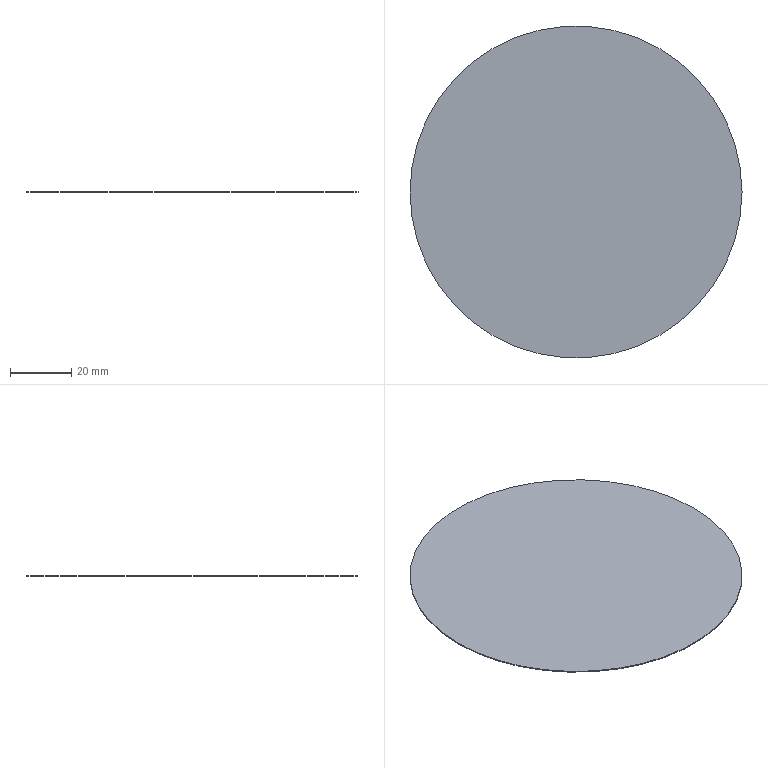Part | SolidWorks | features Extrusion 1 | 1 solid | 4 faces | box 108 x 108 x 0.3 mm | volume 2748 mm3 | cylinder 2 | plane 2 | commonest cylinder face diameters 108 x2
STEP:
#1=CARTESIAN_POINT('',(54.,0.,0.3));
#2=VERTEX_POINT('',#1);
#3=CARTESIAN_POINT('',(-54.,0.,0.3));
#4=VERTEX_POINT('',#3);
#5=CARTESIAN_POINT('',(0.,0.,0.3));
#6=DIRECTION('',(0.,0.,1.));
#7=DIRECTION('',(1.,0.,0.));
#8=AXIS2_PLACEMENT_3D('',#5,#6,#7);
#9=CIRCLE('',#8,54.);
#10=EDGE_CURVE('',#2,#4,#9,.T.);
#11=ORIENTED_EDGE('',*,*,#10,.F.);
#12=CARTESIAN_POINT('',(54.,0.,0.));
#13=VERTEX_POINT('',#12);
#14=CARTESIAN_POINT('',(54.,0.,0.3));
#15=DIRECTION('',(0.,0.,-1.));
#16=VECTOR('',#15,1000.);
#17=LINE('',#14,#16);
#18=EDGE_CURVE('',#2,#13,#17,.T.);
#19=ORIENTED_EDGE('',*,*,#18,.T.);
#20=CARTESIAN_POINT('',(-54.,0.,0.));
#21=VERTEX_POINT('',#20);
#22=CARTESIAN_POINT('',(0.,0.,0.));
#23=DIRECTION('',(0.,0.,1.));
#24=DIRECTION('',(1.,0.,0.));
#25=AXIS2_PLACEMENT_3D('',#22,#23,#24);
#26=CIRCLE('',#25,54.);
#27=EDGE_CURVE('',#13,#21,#26,.T.);
#28=ORIENTED_EDGE('',*,*,#27,.T.);
#29=CARTESIAN_POINT('',(-54.,0.,0.3));
#30=DIRECTION('',(0.,0.,-1.));
#31=VECTOR('',#30,1000.);
#32=LINE('',#29,#31);
#33=EDGE_CURVE('',#4,#21,#32,.T.);
#34=ORIENTED_EDGE('',*,*,#33,.F.);
#35=EDGE_LOOP('',(#11,#19,#28,#34));
#36=FACE_OUTER_BOUND('',#35,.T.);
#37=CARTESIAN_POINT('',(0.,0.,0.3));
#38=DIRECTION('',(0.,0.,-1.));
#39=DIRECTION('',(-1.,0.,0.));
#40=AXIS2_PLACEMENT_3D('',#37,#38,#39);
#41=CYLINDRICAL_SURFACE('',#40,54.);
#42=ADVANCED_FACE('',(#36),#41,.T.);
#43=ORIENTED_EDGE('',*,*,#18,.F.);
#44=CARTESIAN_POINT('',(0.,0.,0.3));
#45=DIRECTION('',(0.,0.,1.));
#46=DIRECTION('',(1.,0.,0.));
#47=AXIS2_PLACEMENT_3D('',#44,#45,#46);
#48=CIRCLE('',#47,54.);
#49=EDGE_CURVE('',#4,#2,#48,.T.);
#50=ORIENTED_EDGE('',*,*,#49,.F.);
#51=ORIENTED_EDGE('',*,*,#33,.T.);
#52=CARTESIAN_POINT('',(0.,0.,0.));
#53=DIRECTION('',(0.,0.,1.));
#54=DIRECTION('',(1.,0.,0.));
#55=AXIS2_PLACEMENT_3D('',#52,#53,#54);
#56=CIRCLE('',#55,54.);
#57=EDGE_CURVE('',#21,#13,#56,.T.);
#58=ORIENTED_EDGE('',*,*,#57,.T.);
#59=EDGE_LOOP('',(#43,#50,#51,#58));
#60=FACE_OUTER_BOUND('',#59,.T.);
#61=CARTESIAN_POINT('',(0.,0.,0.3));
#62=DIRECTION('',(0.,0.,-1.));
#63=DIRECTION('',(-1.,0.,0.));
#64=AXIS2_PLACEMENT_3D('',#61,#62,#63);
#65=CYLINDRICAL_SURFACE('',#64,54.);
#66=ADVANCED_FACE('',(#60),#65,.T.);
#67=ORIENTED_EDGE('',*,*,#49,.T.);
#68=ORIENTED_EDGE('',*,*,#10,.T.);
#69=EDGE_LOOP('',(#67,#68));
#70=FACE_OUTER_BOUND('',#69,.T.);
#71=CARTESIAN_POINT('',(0.,0.,0.3));
#72=DIRECTION('',(0.,0.,1.));
#73=DIRECTION('',(1.,0.,0.));
#74=AXIS2_PLACEMENT_3D('',#71,#72,#73);
#75=PLANE('',#74);
#76=ADVANCED_FACE('',(#70),#75,.T.);
#77=ORIENTED_EDGE('',*,*,#57,.F.);
#78=ORIENTED_EDGE('',*,*,#27,.F.);
#79=EDGE_LOOP('',(#77,#78));
#80=FACE_OUTER_BOUND('',#79,.T.);
#81=CARTESIAN_POINT('',(0.,0.,0.));
#82=DIRECTION('',(0.,0.,1.));
#83=DIRECTION('',(1.,0.,0.));
#84=AXIS2_PLACEMENT_3D('',#81,#82,#83);
#85=PLANE('',#84);
#86=ADVANCED_FACE('',(#80),#85,.F.);
#87=CLOSED_SHELL('',(#42,#66,#76,#86));
#88=MANIFOLD_SOLID_BREP('',#87);
#89=CARTESIAN_POINT('',(0.,0.,0.));
#90=DIRECTION('',(0.,0.,1.));
#91=DIRECTION('',(1.,0.,0.));
#92=AXIS2_PLACEMENT_3D('',#89,#90,#91);
#93=(LENGTH_UNIT()NAMED_UNIT(*)SI_UNIT(.MILLI.,.METRE.));
#94=UNCERTAINTY_MEASURE_WITH_UNIT(LENGTH_MEASURE(0.00001),#93,'','');
#95=(NAMED_UNIT(*)PLANE_ANGLE_UNIT()SI_UNIT($,.RADIAN.));
#96=(NAMED_UNIT(*)SI_UNIT($,.STERADIAN.)SOLID_ANGLE_UNIT());
#97=(GEOMETRIC_REPRESENTATION_CONTEXT(3)GLOBAL_UNCERTAINTY_ASSIGNED_CONTEXT((#94))GLOBAL_UNIT_ASSIGNED_CONTEXT((#93,#95,#96))REPRESENTATION_CONTEXT('',''));
#98=ADVANCED_BREP_SHAPE_REPRESENTATION('',(#88,#92),#97);